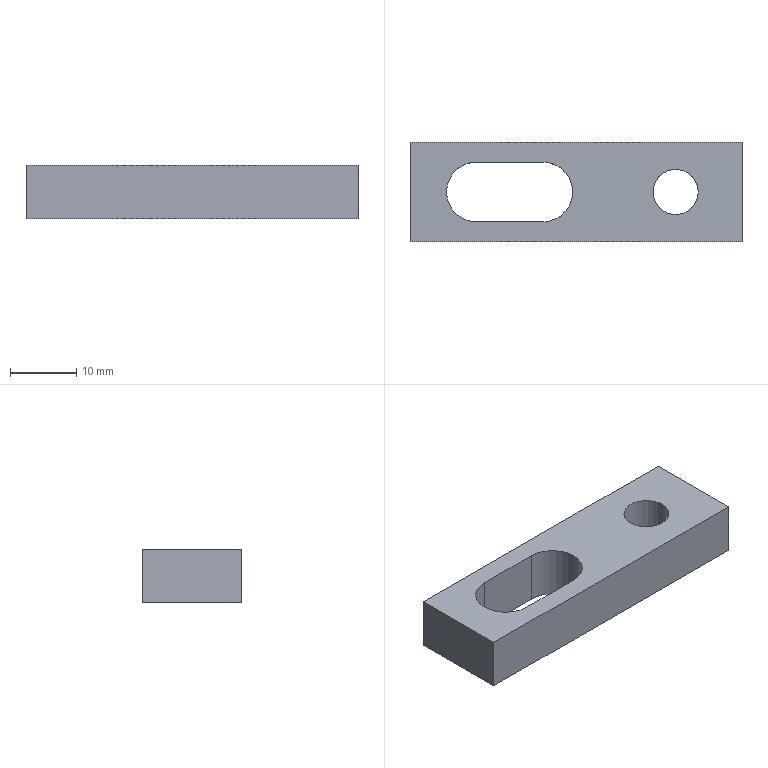Part | STEP file | Tensioning adjustment block QY-1-11 | 1 solid | 13 faces | box 50 x 15 x 8 mm | volume 4481 mm3 | plane 8 | cylinder 5 | commonest cylinder face diameters 9 x3 6.8 x2
STEP:
#1=CARTESIAN_POINT('',(0.,0.,0.));
#2=DIRECTION('',(0.,0.,1.));
#3=DIRECTION('',(1.,0.,0.));
#4=AXIS2_PLACEMENT_3D('',#1,#2,#3);
#5=CARTESIAN_POINT('',(-5.,4.5,0.));
#6=VERTEX_POINT('',#5);
#7=CARTESIAN_POINT('',(-5.,4.5,8.));
#8=VERTEX_POINT('',#7);
#9=CARTESIAN_POINT('',(-5.,4.5,0.));
#10=DIRECTION('',(0.,0.,1.));
#11=VECTOR('',#10,1.);
#12=LINE('',#9,#11);
#13=CARTESIAN_POINT('',(-5.,0.,0.));
#14=DIRECTION('',(0.,0.,1.));
#15=DIRECTION('',(1.,0.,0.));
#16=AXIS2_PLACEMENT_3D('',#13,#14,#15);
#17=CYLINDRICAL_SURFACE('',#16,4.5);
#18=CARTESIAN_POINT('',(1.571,0.));
#19=DIRECTION('',(0.,1.));
#20=VECTOR('',#19,1.);
#21=LINE('',#18,#20);
#22=(GEOMETRIC_REPRESENTATION_CONTEXT(2)PARAMETRIC_REPRESENTATION_CONTEXT()REPRESENTATION_CONTEXT('',''));
#23=DEFINITIONAL_REPRESENTATION('',(#21),#22);
#24=PCURVE('',#17,#23);
#25=CARTESIAN_POINT('',(-15.,4.5,0.));
#26=DIRECTION('',(0.,1.,0.));
#27=DIRECTION('',(-1.,0.,0.));
#28=AXIS2_PLACEMENT_3D('',#25,#26,#27);
#29=PLANE('',#28);
#30=CARTESIAN_POINT('',(-10.,0.));
#31=DIRECTION('',(0.,1.));
#32=VECTOR('',#31,1.);
#33=LINE('',#30,#32);
#34=(GEOMETRIC_REPRESENTATION_CONTEXT(2)PARAMETRIC_REPRESENTATION_CONTEXT()REPRESENTATION_CONTEXT('',''));
#35=DEFINITIONAL_REPRESENTATION('',(#33),#34);
#36=PCURVE('',#29,#35);
#37=SURFACE_CURVE('',#12,(#24,#36),.PCURVE_S1.);
#38=EDGE_CURVE('',#6,#8,#37,.T.);
#39=ORIENTED_EDGE('',*,*,#38,.T.);
#40=CARTESIAN_POINT('',(-0.5,0.,8.));
#41=VERTEX_POINT('',#40);
#42=CARTESIAN_POINT('',(-5.,0.,8.));
#43=DIRECTION('',(0.,0.,1.));
#44=DIRECTION('',(1.,0.,0.));
#45=AXIS2_PLACEMENT_3D('',#42,#43,#44);
#46=CIRCLE('',#45,4.5);
#47=CARTESIAN_POINT('',(0.,8.));
#48=DIRECTION('',(1.,0.));
#49=VECTOR('',#48,1.);
#50=LINE('',#47,#49);
#51=(GEOMETRIC_REPRESENTATION_CONTEXT(2)PARAMETRIC_REPRESENTATION_CONTEXT()REPRESENTATION_CONTEXT('',''));
#52=DEFINITIONAL_REPRESENTATION('',(#50),#51);
#53=PCURVE('',#17,#52);
#54=CARTESIAN_POINT('',(0.,0.,8.));
#55=DIRECTION('',(0.,0.,1.));
#56=DIRECTION('',(1.,0.,0.));
#57=AXIS2_PLACEMENT_3D('',#54,#55,#56);
#58=PLANE('',#57);
#59=CARTESIAN_POINT('',(-5.,0.));
#60=DIRECTION('',(1.,0.));
#61=AXIS2_PLACEMENT_2D('',#59,#60);
#62=CIRCLE('',#61,4.5);
#63=(GEOMETRIC_REPRESENTATION_CONTEXT(2)PARAMETRIC_REPRESENTATION_CONTEXT()REPRESENTATION_CONTEXT('',''));
#64=DEFINITIONAL_REPRESENTATION('',(#62),#63);
#65=PCURVE('',#58,#64);
#66=SURFACE_CURVE('',#46,(#53,#65),.PCURVE_S1.);
#67=EDGE_CURVE('',#41,#8,#66,.T.);
#68=ORIENTED_EDGE('',*,*,#67,.F.);
#69=CARTESIAN_POINT('',(-0.5,0.,0.));
#70=VERTEX_POINT('',#69);
#71=CARTESIAN_POINT('',(-0.5,0.,0.));
#72=DIRECTION('',(0.,0.,1.));
#73=VECTOR('',#72,1.);
#74=LINE('',#71,#73);
#75=CARTESIAN_POINT('',(0.,0.));
#76=DIRECTION('',(0.,1.));
#77=VECTOR('',#76,1.);
#78=LINE('',#75,#77);
#79=(GEOMETRIC_REPRESENTATION_CONTEXT(2)PARAMETRIC_REPRESENTATION_CONTEXT()REPRESENTATION_CONTEXT('',''));
#80=DEFINITIONAL_REPRESENTATION('',(#78),#79);
#81=PCURVE('',#17,#80);
#82=CARTESIAN_POINT('',(-5.,0.,0.));
#83=DIRECTION('',(0.,0.,1.));
#84=DIRECTION('',(1.,0.,0.));
#85=AXIS2_PLACEMENT_3D('',#82,#83,#84);
#86=CYLINDRICAL_SURFACE('',#85,4.5);
#87=CARTESIAN_POINT('',(6.283,0.));
#88=DIRECTION('',(0.,1.));
#89=VECTOR('',#88,1.);
#90=LINE('',#87,#89);
#91=(GEOMETRIC_REPRESENTATION_CONTEXT(2)PARAMETRIC_REPRESENTATION_CONTEXT()REPRESENTATION_CONTEXT('',''));
#92=DEFINITIONAL_REPRESENTATION('',(#90),#91);
#93=PCURVE('',#86,#92);
#94=SURFACE_CURVE('',#74,(#81,#93),.PCURVE_S1.);
#95=EDGE_CURVE('',#70,#41,#94,.T.);
#96=ORIENTED_EDGE('',*,*,#95,.F.);
#97=CARTESIAN_POINT('',(-5.,0.,0.));
#98=DIRECTION('',(0.,0.,1.));
#99=DIRECTION('',(1.,0.,0.));
#100=AXIS2_PLACEMENT_3D('',#97,#98,#99);
#101=CIRCLE('',#100,4.5);
#102=CARTESIAN_POINT('',(0.,0.));
#103=DIRECTION('',(1.,0.));
#104=VECTOR('',#103,1.);
#105=LINE('',#102,#104);
#106=(GEOMETRIC_REPRESENTATION_CONTEXT(2)PARAMETRIC_REPRESENTATION_CONTEXT()REPRESENTATION_CONTEXT('',''));
#107=DEFINITIONAL_REPRESENTATION('',(#105),#106);
#108=PCURVE('',#17,#107);
#109=CARTESIAN_POINT('',(0.,0.,0.));
#110=DIRECTION('',(0.,0.,1.));
#111=DIRECTION('',(1.,0.,0.));
#112=AXIS2_PLACEMENT_3D('',#109,#110,#111);
#113=PLANE('',#112);
#114=CARTESIAN_POINT('',(-5.,0.));
#115=DIRECTION('',(1.,0.));
#116=AXIS2_PLACEMENT_2D('',#114,#115);
#117=CIRCLE('',#116,4.5);
#118=(GEOMETRIC_REPRESENTATION_CONTEXT(2)PARAMETRIC_REPRESENTATION_CONTEXT()REPRESENTATION_CONTEXT('',''));
#119=DEFINITIONAL_REPRESENTATION('',(#117),#118);
#120=PCURVE('',#113,#119);
#121=SURFACE_CURVE('',#101,(#108,#120),.PCURVE_S1.);
#122=EDGE_CURVE('',#70,#6,#121,.T.);
#123=ORIENTED_EDGE('',*,*,#122,.T.);
#124=EDGE_LOOP('',(#39,#68,#96,#123));
#125=FACE_BOUND('',#124,.F.);
#126=ADVANCED_FACE('',(#125),#17,.F.);
#127=CARTESIAN_POINT('',(18.4,0.,0.));
#128=VERTEX_POINT('',#127);
#129=CARTESIAN_POINT('',(18.4,0.,8.));
#130=VERTEX_POINT('',#129);
#131=CARTESIAN_POINT('',(18.4,0.,8.));
#132=DIRECTION('',(0.,0.,1.));
#133=VECTOR('',#132,1.);
#134=LINE('',#131,#133);
#135=CARTESIAN_POINT('',(15.,0.,8.));
#136=DIRECTION('',(0.,0.,1.));
#137=DIRECTION('',(1.,0.,0.));
#138=AXIS2_PLACEMENT_3D('',#135,#136,#137);
#139=CYLINDRICAL_SURFACE('',#138,3.4);
#140=CARTESIAN_POINT('',(6.283,0.));
#141=DIRECTION('',(0.,1.));
#142=VECTOR('',#141,1.);
#143=LINE('',#140,#142);
#144=(GEOMETRIC_REPRESENTATION_CONTEXT(2)PARAMETRIC_REPRESENTATION_CONTEXT()REPRESENTATION_CONTEXT('',''));
#145=DEFINITIONAL_REPRESENTATION('',(#143),#144);
#146=PCURVE('',#139,#145);
#147=CARTESIAN_POINT('',(15.,0.,8.));
#148=DIRECTION('',(0.,0.,1.));
#149=DIRECTION('',(1.,0.,0.));
#150=AXIS2_PLACEMENT_3D('',#147,#148,#149);
#151=CYLINDRICAL_SURFACE('',#150,3.4);
#152=CARTESIAN_POINT('',(0.,0.));
#153=DIRECTION('',(0.,1.));
#154=VECTOR('',#153,1.);
#155=LINE('',#152,#154);
#156=(GEOMETRIC_REPRESENTATION_CONTEXT(2)PARAMETRIC_REPRESENTATION_CONTEXT()REPRESENTATION_CONTEXT('',''));
#157=DEFINITIONAL_REPRESENTATION('',(#155),#156);
#158=PCURVE('',#151,#157);
#159=SURFACE_CURVE('',#134,(#146,#158),.PCURVE_S1.);
#160=EDGE_CURVE('',#128,#130,#159,.T.);
#161=ORIENTED_EDGE('',*,*,#160,.T.);
#162=CARTESIAN_POINT('',(11.6,0.,8.));
#163=VERTEX_POINT('',#162);
#164=CARTESIAN_POINT('',(15.,0.,8.));
#165=DIRECTION('',(0.,0.,1.));
#166=DIRECTION('',(1.,0.,0.));
#167=AXIS2_PLACEMENT_3D('',#164,#165,#166);
#168=CIRCLE('',#167,3.4);
#169=CARTESIAN_POINT('',(0.,0.));
#170=DIRECTION('',(1.,0.));
#171=VECTOR('',#170,1.);
#172=LINE('',#169,#171);
#173=(GEOMETRIC_REPRESENTATION_CONTEXT(2)PARAMETRIC_REPRESENTATION_CONTEXT()REPRESENTATION_CONTEXT('',''));
#174=DEFINITIONAL_REPRESENTATION('',(#172),#173);
#175=PCURVE('',#139,#174);
#176=CARTESIAN_POINT('',(15.,0.));
#177=DIRECTION('',(1.,0.));
#178=AXIS2_PLACEMENT_2D('',#176,#177);
#179=CIRCLE('',#178,3.4);
#180=(GEOMETRIC_REPRESENTATION_CONTEXT(2)PARAMETRIC_REPRESENTATION_CONTEXT()REPRESENTATION_CONTEXT('',''));
#181=DEFINITIONAL_REPRESENTATION('',(#179),#180);
#182=PCURVE('',#58,#181);
#183=SURFACE_CURVE('',#168,(#175,#182),.PCURVE_S1.);
#184=EDGE_CURVE('',#163,#130,#183,.T.);
#185=ORIENTED_EDGE('',*,*,#184,.F.);
#186=CARTESIAN_POINT('',(11.6,0.,0.));
#187=VERTEX_POINT('',#186);
#188=CARTESIAN_POINT('',(11.6,0.,8.));
#189=DIRECTION('',(0.,0.,1.));
#190=VECTOR('',#189,1.);
#191=LINE('',#188,#190);
#192=CARTESIAN_POINT('',(3.142,0.));
#193=DIRECTION('',(0.,1.));
#194=VECTOR('',#193,1.);
#195=LINE('',#192,#194);
#196=(GEOMETRIC_REPRESENTATION_CONTEXT(2)PARAMETRIC_REPRESENTATION_CONTEXT()REPRESENTATION_CONTEXT('',''));
#197=DEFINITIONAL_REPRESENTATION('',(#195),#196);
#198=PCURVE('',#139,#197);
#199=CARTESIAN_POINT('',(3.142,0.));
#200=DIRECTION('',(0.,1.));
#201=VECTOR('',#200,1.);
#202=LINE('',#199,#201);
#203=(GEOMETRIC_REPRESENTATION_CONTEXT(2)PARAMETRIC_REPRESENTATION_CONTEXT()REPRESENTATION_CONTEXT('',''));
#204=DEFINITIONAL_REPRESENTATION('',(#202),#203);
#205=PCURVE('',#151,#204);
#206=SURFACE_CURVE('',#191,(#198,#205),.PCURVE_S1.);
#207=EDGE_CURVE('',#187,#163,#206,.T.);
#208=ORIENTED_EDGE('',*,*,#207,.F.);
#209=CARTESIAN_POINT('',(15.,0.,0.));
#210=DIRECTION('',(0.,0.,1.));
#211=DIRECTION('',(1.,0.,0.));
#212=AXIS2_PLACEMENT_3D('',#209,#210,#211);
#213=CIRCLE('',#212,3.4);
#214=CARTESIAN_POINT('',(0.,-8.));
#215=DIRECTION('',(1.,0.));
#216=VECTOR('',#215,1.);
#217=LINE('',#214,#216);
#218=(GEOMETRIC_REPRESENTATION_CONTEXT(2)PARAMETRIC_REPRESENTATION_CONTEXT()REPRESENTATION_CONTEXT('',''));
#219=DEFINITIONAL_REPRESENTATION('',(#217),#218);
#220=PCURVE('',#139,#219);
#221=CARTESIAN_POINT('',(15.,0.));
#222=DIRECTION('',(1.,0.));
#223=AXIS2_PLACEMENT_2D('',#221,#222);
#224=CIRCLE('',#223,3.4);
#225=(GEOMETRIC_REPRESENTATION_CONTEXT(2)PARAMETRIC_REPRESENTATION_CONTEXT()REPRESENTATION_CONTEXT('',''));
#226=DEFINITIONAL_REPRESENTATION('',(#224),#225);
#227=PCURVE('',#113,#226);
#228=SURFACE_CURVE('',#213,(#220,#227),.PCURVE_S1.);
#229=EDGE_CURVE('',#187,#128,#228,.T.);
#230=ORIENTED_EDGE('',*,*,#229,.T.);
#231=EDGE_LOOP('',(#161,#185,#208,#230));
#232=FACE_BOUND('',#231,.F.);
#233=ADVANCED_FACE('',(#232),#139,.F.);
#234=CARTESIAN_POINT('',(25.,-7.5,0.));
#235=VERTEX_POINT('',#234);
#236=CARTESIAN_POINT('',(25.,7.5,0.));
#237=VERTEX_POINT('',#236);
#238=CARTESIAN_POINT('',(25.,7.5,0.));
#239=DIRECTION('',(0.,1.,0.));
#240=VECTOR('',#239,1.);
#241=LINE('',#238,#240);
#242=CARTESIAN_POINT('',(25.,7.5,8.));
#243=DIRECTION('',(-1.,0.,0.));
#244=DIRECTION('',(0.,0.,1.));
#245=AXIS2_PLACEMENT_3D('',#242,#243,#244);
#246=PLANE('',#245);
#247=CARTESIAN_POINT('',(-8.,0.));
#248=DIRECTION('',(0.,1.));
#249=VECTOR('',#248,1.);
#250=LINE('',#247,#249);
#251=(GEOMETRIC_REPRESENTATION_CONTEXT(2)PARAMETRIC_REPRESENTATION_CONTEXT()REPRESENTATION_CONTEXT('',''));
#252=DEFINITIONAL_REPRESENTATION('',(#250),#251);
#253=PCURVE('',#246,#252);
#254=CARTESIAN_POINT('',(25.,7.5));
#255=DIRECTION('',(0.,1.));
#256=VECTOR('',#255,1.);
#257=LINE('',#254,#256);
#258=(GEOMETRIC_REPRESENTATION_CONTEXT(2)PARAMETRIC_REPRESENTATION_CONTEXT()REPRESENTATION_CONTEXT('',''));
#259=DEFINITIONAL_REPRESENTATION('',(#257),#258);
#260=PCURVE('',#113,#259);
#261=SURFACE_CURVE('',#241,(#253,#260),.PCURVE_S1.);
#262=EDGE_CURVE('',#235,#237,#261,.T.);
#263=ORIENTED_EDGE('',*,*,#262,.T.);
#264=CARTESIAN_POINT('',(25.,7.5,8.));
#265=VERTEX_POINT('',#264);
#266=CARTESIAN_POINT('',(25.,7.5,8.));
#267=DIRECTION('',(0.,0.,-1.));
#268=VECTOR('',#267,1.);
#269=LINE('',#266,#268);
#270=CARTESIAN_POINT('',(0.,0.));
#271=DIRECTION('',(-1.,0.));
#272=VECTOR('',#271,1.);
#273=LINE('',#270,#272);
#274=(GEOMETRIC_REPRESENTATION_CONTEXT(2)PARAMETRIC_REPRESENTATION_CONTEXT()REPRESENTATION_CONTEXT('',''));
#275=DEFINITIONAL_REPRESENTATION('',(#273),#274);
#276=PCURVE('',#246,#275);
#277=CARTESIAN_POINT('',(-25.,7.5,8.));
#278=DIRECTION('',(0.,-1.,0.));
#279=DIRECTION('',(0.,0.,-1.));
#280=AXIS2_PLACEMENT_3D('',#277,#278,#279);
#281=PLANE('',#280);
#282=CARTESIAN_POINT('',(0.,50.));
#283=DIRECTION('',(1.,0.));
#284=VECTOR('',#283,1.);
#285=LINE('',#282,#284);
#286=(GEOMETRIC_REPRESENTATION_CONTEXT(2)PARAMETRIC_REPRESENTATION_CONTEXT()REPRESENTATION_CONTEXT('',''));
#287=DEFINITIONAL_REPRESENTATION('',(#285),#286);
#288=PCURVE('',#281,#287);
#289=SURFACE_CURVE('',#269,(#276,#288),.PCURVE_S1.);
#290=EDGE_CURVE('',#265,#237,#289,.T.);
#291=ORIENTED_EDGE('',*,*,#290,.F.);
#292=CARTESIAN_POINT('',(25.,-7.5,8.));
#293=VERTEX_POINT('',#292);
#294=CARTESIAN_POINT('',(25.,7.5,8.));
#295=DIRECTION('',(0.,1.,0.));
#296=VECTOR('',#295,1.);
#297=LINE('',#294,#296);
#298=CARTESIAN_POINT('',(0.,0.));
#299=DIRECTION('',(0.,1.));
#300=VECTOR('',#299,1.);
#301=LINE('',#298,#300);
#302=(GEOMETRIC_REPRESENTATION_CONTEXT(2)PARAMETRIC_REPRESENTATION_CONTEXT()REPRESENTATION_CONTEXT('',''));
#303=DEFINITIONAL_REPRESENTATION('',(#301),#302);
#304=PCURVE('',#246,#303);
#305=CARTESIAN_POINT('',(25.,7.5));
#306=DIRECTION('',(0.,1.));
#307=VECTOR('',#306,1.);
#308=LINE('',#305,#307);
#309=(GEOMETRIC_REPRESENTATION_CONTEXT(2)PARAMETRIC_REPRESENTATION_CONTEXT()REPRESENTATION_CONTEXT('',''));
#310=DEFINITIONAL_REPRESENTATION('',(#308),#309);
#311=PCURVE('',#58,#310);
#312=SURFACE_CURVE('',#297,(#304,#311),.PCURVE_S1.);
#313=EDGE_CURVE('',#293,#265,#312,.T.);
#314=ORIENTED_EDGE('',*,*,#313,.F.);
#315=CARTESIAN_POINT('',(25.,-7.5,8.));
#316=DIRECTION('',(0.,0.,-1.));
#317=VECTOR('',#316,1.);
#318=LINE('',#315,#317);
#319=CARTESIAN_POINT('',(0.,-15.));
#320=DIRECTION('',(-1.,0.));
#321=VECTOR('',#320,1.);
#322=LINE('',#319,#321);
#323=(GEOMETRIC_REPRESENTATION_CONTEXT(2)PARAMETRIC_REPRESENTATION_CONTEXT()REPRESENTATION_CONTEXT('',''));
#324=DEFINITIONAL_REPRESENTATION('',(#322),#323);
#325=PCURVE('',#246,#324);
#326=CARTESIAN_POINT('',(-25.,-7.5,8.));
#327=DIRECTION('',(0.,1.,0.));
#328=DIRECTION('',(0.,0.,1.));
#329=AXIS2_PLACEMENT_3D('',#326,#327,#328);
#330=PLANE('',#329);
#331=CARTESIAN_POINT('',(0.,50.));
#332=DIRECTION('',(-1.,0.));
#333=VECTOR('',#332,1.);
#334=LINE('',#331,#333);
#335=(GEOMETRIC_REPRESENTATION_CONTEXT(2)PARAMETRIC_REPRESENTATION_CONTEXT()REPRESENTATION_CONTEXT('',''));
#336=DEFINITIONAL_REPRESENTATION('',(#334),#335);
#337=PCURVE('',#330,#336);
#338=SURFACE_CURVE('',#318,(#325,#337),.PCURVE_S1.);
#339=EDGE_CURVE('',#293,#235,#338,.T.);
#340=ORIENTED_EDGE('',*,*,#339,.T.);
#341=EDGE_LOOP('',(#263,#291,#314,#340));
#342=FACE_BOUND('',#341,.T.);
#343=ADVANCED_FACE('',(#342),#246,.F.);
#344=CARTESIAN_POINT('',(-25.,7.5,0.));
#345=VERTEX_POINT('',#344);
#346=CARTESIAN_POINT('',(-25.,7.5,0.));
#347=DIRECTION('',(-1.,0.,0.));
#348=VECTOR('',#347,1.);
#349=LINE('',#346,#348);
#350=CARTESIAN_POINT('',(8.,0.));
#351=DIRECTION('',(0.,-1.));
#352=VECTOR('',#351,1.);
#353=LINE('',#350,#352);
#354=(GEOMETRIC_REPRESENTATION_CONTEXT(2)PARAMETRIC_REPRESENTATION_CONTEXT()REPRESENTATION_CONTEXT('',''));
#355=DEFINITIONAL_REPRESENTATION('',(#353),#354);
#356=PCURVE('',#281,#355);
#357=CARTESIAN_POINT('',(-25.,7.5));
#358=DIRECTION('',(-1.,0.));
#359=VECTOR('',#358,1.);
#360=LINE('',#357,#359);
#361=(GEOMETRIC_REPRESENTATION_CONTEXT(2)PARAMETRIC_REPRESENTATION_CONTEXT()REPRESENTATION_CONTEXT('',''));
#362=DEFINITIONAL_REPRESENTATION('',(#360),#361);
#363=PCURVE('',#113,#362);
#364=SURFACE_CURVE('',#349,(#356,#363),.PCURVE_S1.);
#365=EDGE_CURVE('',#237,#345,#364,.T.);
#366=ORIENTED_EDGE('',*,*,#365,.T.);
#367=CARTESIAN_POINT('',(-25.,7.5,8.));
#368=VERTEX_POINT('',#367);
#369=CARTESIAN_POINT('',(-25.,7.5,8.));
#370=DIRECTION('',(0.,0.,-1.));
#371=VECTOR('',#370,1.);
#372=LINE('',#369,#371);
#373=CARTESIAN_POINT('',(0.,0.));
#374=DIRECTION('',(1.,0.));
#375=VECTOR('',#374,1.);
#376=LINE('',#373,#375);
#377=(GEOMETRIC_REPRESENTATION_CONTEXT(2)PARAMETRIC_REPRESENTATION_CONTEXT()REPRESENTATION_CONTEXT('',''));
#378=DEFINITIONAL_REPRESENTATION('',(#376),#377);
#379=PCURVE('',#281,#378);
#380=CARTESIAN_POINT('',(-25.,7.5,8.));
#381=DIRECTION('',(1.,0.,0.));
#382=DIRECTION('',(0.,0.,-1.));
#383=AXIS2_PLACEMENT_3D('',#380,#381,#382);
#384=PLANE('',#383);
#385=CARTESIAN_POINT('',(0.,0.));
#386=DIRECTION('',(1.,0.));
#387=VECTOR('',#386,1.);
#388=LINE('',#385,#387);
#389=(GEOMETRIC_REPRESENTATION_CONTEXT(2)PARAMETRIC_REPRESENTATION_CONTEXT()REPRESENTATION_CONTEXT('',''));
#390=DEFINITIONAL_REPRESENTATION('',(#388),#389);
#391=PCURVE('',#384,#390);
#392=SURFACE_CURVE('',#372,(#379,#391),.PCURVE_S1.);
#393=EDGE_CURVE('',#368,#345,#392,.T.);
#394=ORIENTED_EDGE('',*,*,#393,.F.);
#395=CARTESIAN_POINT('',(-25.,7.5,8.));
#396=DIRECTION('',(-1.,0.,0.));
#397=VECTOR('',#396,1.);
#398=LINE('',#395,#397);
#399=CARTESIAN_POINT('',(0.,0.));
#400=DIRECTION('',(0.,-1.));
#401=VECTOR('',#400,1.);
#402=LINE('',#399,#401);
#403=(GEOMETRIC_REPRESENTATION_CONTEXT(2)PARAMETRIC_REPRESENTATION_CONTEXT()REPRESENTATION_CONTEXT('',''));
#404=DEFINITIONAL_REPRESENTATION('',(#402),#403);
#405=PCURVE('',#281,#404);
#406=CARTESIAN_POINT('',(-25.,7.5));
#407=DIRECTION('',(-1.,0.));
#408=VECTOR('',#407,1.);
#409=LINE('',#406,#408);
#410=(GEOMETRIC_REPRESENTATION_CONTEXT(2)PARAMETRIC_REPRESENTATION_CONTEXT()REPRESENTATION_CONTEXT('',''));
#411=DEFINITIONAL_REPRESENTATION('',(#409),#410);
#412=PCURVE('',#58,#411);
#413=SURFACE_CURVE('',#398,(#405,#412),.PCURVE_S1.);
#414=EDGE_CURVE('',#265,#368,#413,.T.);
#415=ORIENTED_EDGE('',*,*,#414,.F.);
#416=ORIENTED_EDGE('',*,*,#290,.T.);
#417=EDGE_LOOP('',(#366,#394,#415,#416));
#418=FACE_BOUND('',#417,.T.);
#419=ADVANCED_FACE('',(#418),#281,.F.);
#420=CARTESIAN_POINT('',(-25.,-7.5,0.));
#421=VERTEX_POINT('',#420);
#422=CARTESIAN_POINT('',(-25.,7.5,0.));
#423=DIRECTION('',(0.,-1.,0.));
#424=VECTOR('',#423,1.);
#425=LINE('',#422,#424);
#426=CARTESIAN_POINT('',(8.,0.));
#427=DIRECTION('',(0.,-1.));
#428=VECTOR('',#427,1.);
#429=LINE('',#426,#428);
#430=(GEOMETRIC_REPRESENTATION_CONTEXT(2)PARAMETRIC_REPRESENTATION_CONTEXT()REPRESENTATION_CONTEXT('',''));
#431=DEFINITIONAL_REPRESENTATION('',(#429),#430);
#432=PCURVE('',#384,#431);
#433=CARTESIAN_POINT('',(-25.,7.5));
#434=DIRECTION('',(0.,-1.));
#435=VECTOR('',#434,1.);
#436=LINE('',#433,#435);
#437=(GEOMETRIC_REPRESENTATION_CONTEXT(2)PARAMETRIC_REPRESENTATION_CONTEXT()REPRESENTATION_CONTEXT('',''));
#438=DEFINITIONAL_REPRESENTATION('',(#436),#437);
#439=PCURVE('',#113,#438);
#440=SURFACE_CURVE('',#425,(#432,#439),.PCURVE_S1.);
#441=EDGE_CURVE('',#345,#421,#440,.T.);
#442=ORIENTED_EDGE('',*,*,#441,.T.);
#443=CARTESIAN_POINT('',(-25.,-7.5,8.));
#444=VERTEX_POINT('',#443);
#445=CARTESIAN_POINT('',(-25.,-7.5,8.));
#446=DIRECTION('',(0.,0.,-1.));
#447=VECTOR('',#446,1.);
#448=LINE('',#445,#447);
#449=CARTESIAN_POINT('',(0.,-15.));
#450=DIRECTION('',(1.,0.));
#451=VECTOR('',#450,1.);
#452=LINE('',#449,#451);
#453=(GEOMETRIC_REPRESENTATION_CONTEXT(2)PARAMETRIC_REPRESENTATION_CONTEXT()REPRESENTATION_CONTEXT('',''));
#454=DEFINITIONAL_REPRESENTATION('',(#452),#453);
#455=PCURVE('',#384,#454);
#456=CARTESIAN_POINT('',(0.,0.));
#457=DIRECTION('',(-1.,0.));
#458=VECTOR('',#457,1.);
#459=LINE('',#456,#458);
#460=(GEOMETRIC_REPRESENTATION_CONTEXT(2)PARAMETRIC_REPRESENTATION_CONTEXT()REPRESENTATION_CONTEXT('',''));
#461=DEFINITIONAL_REPRESENTATION('',(#459),#460);
#462=PCURVE('',#330,#461);
#463=SURFACE_CURVE('',#448,(#455,#462),.PCURVE_S1.);
#464=EDGE_CURVE('',#444,#421,#463,.T.);
#465=ORIENTED_EDGE('',*,*,#464,.F.);
#466=CARTESIAN_POINT('',(-25.,7.5,8.));
#467=DIRECTION('',(0.,-1.,0.));
#468=VECTOR('',#467,1.);
#469=LINE('',#466,#468);
#470=CARTESIAN_POINT('',(0.,0.));
#471=DIRECTION('',(0.,-1.));
#472=VECTOR('',#471,1.);
#473=LINE('',#470,#472);
#474=(GEOMETRIC_REPRESENTATION_CONTEXT(2)PARAMETRIC_REPRESENTATION_CONTEXT()REPRESENTATION_CONTEXT('',''));
#475=DEFINITIONAL_REPRESENTATION('',(#473),#474);
#476=PCURVE('',#384,#475);
#477=CARTESIAN_POINT('',(-25.,7.5));
#478=DIRECTION('',(0.,-1.));
#479=VECTOR('',#478,1.);
#480=LINE('',#477,#479);
#481=(GEOMETRIC_REPRESENTATION_CONTEXT(2)PARAMETRIC_REPRESENTATION_CONTEXT()REPRESENTATION_CONTEXT('',''));
#482=DEFINITIONAL_REPRESENTATION('',(#480),#481);
#483=PCURVE('',#58,#482);
#484=SURFACE_CURVE('',#469,(#476,#483),.PCURVE_S1.);
#485=EDGE_CURVE('',#368,#444,#484,.T.);
#486=ORIENTED_EDGE('',*,*,#485,.F.);
#487=ORIENTED_EDGE('',*,*,#393,.T.);
#488=EDGE_LOOP('',(#442,#465,#486,#487));
#489=FACE_BOUND('',#488,.T.);
#490=ADVANCED_FACE('',(#489),#384,.F.);
#491=CARTESIAN_POINT('',(-25.,-7.5,0.));
#492=DIRECTION('',(1.,0.,0.));
#493=VECTOR('',#492,1.);
#494=LINE('',#491,#493);
#495=CARTESIAN_POINT('',(-8.,0.));
#496=DIRECTION('',(0.,1.));
#497=VECTOR('',#496,1.);
#498=LINE('',#495,#497);
#499=(GEOMETRIC_REPRESENTATION_CONTEXT(2)PARAMETRIC_REPRESENTATION_CONTEXT()REPRESENTATION_CONTEXT('',''));
#500=DEFINITIONAL_REPRESENTATION('',(#498),#499);
#501=PCURVE('',#330,#500);
#502=CARTESIAN_POINT('',(-25.,-7.5));
#503=DIRECTION('',(1.,0.));
#504=VECTOR('',#503,1.);
#505=LINE('',#502,#504);
#506=(GEOMETRIC_REPRESENTATION_CONTEXT(2)PARAMETRIC_REPRESENTATION_CONTEXT()REPRESENTATION_CONTEXT('',''));
#507=DEFINITIONAL_REPRESENTATION('',(#505),#506);
#508=PCURVE('',#113,#507);
#509=SURFACE_CURVE('',#494,(#501,#508),.PCURVE_S1.);
#510=EDGE_CURVE('',#421,#235,#509,.T.);
#511=ORIENTED_EDGE('',*,*,#510,.T.);
#512=ORIENTED_EDGE('',*,*,#339,.F.);
#513=CARTESIAN_POINT('',(-25.,-7.5,8.));
#514=DIRECTION('',(1.,0.,0.));
#515=VECTOR('',#514,1.);
#516=LINE('',#513,#515);
#517=CARTESIAN_POINT('',(0.,0.));
#518=DIRECTION('',(0.,1.));
#519=VECTOR('',#518,1.);
#520=LINE('',#517,#519);
#521=(GEOMETRIC_REPRESENTATION_CONTEXT(2)PARAMETRIC_REPRESENTATION_CONTEXT()REPRESENTATION_CONTEXT('',''));
#522=DEFINITIONAL_REPRESENTATION('',(#520),#521);
#523=PCURVE('',#330,#522);
#524=CARTESIAN_POINT('',(-25.,-7.5));
#525=DIRECTION('',(1.,0.));
#526=VECTOR('',#525,1.);
#527=LINE('',#524,#526);
#528=(GEOMETRIC_REPRESENTATION_CONTEXT(2)PARAMETRIC_REPRESENTATION_CONTEXT()REPRESENTATION_CONTEXT('',''));
#529=DEFINITIONAL_REPRESENTATION('',(#527),#528);
#530=PCURVE('',#58,#529);
#531=SURFACE_CURVE('',#516,(#523,#530),.PCURVE_S1.);
#532=EDGE_CURVE('',#444,#293,#531,.T.);
#533=ORIENTED_EDGE('',*,*,#532,.F.);
#534=ORIENTED_EDGE('',*,*,#464,.T.);
#535=EDGE_LOOP('',(#511,#512,#533,#534));
#536=FACE_BOUND('',#535,.T.);
#537=ADVANCED_FACE('',(#536),#330,.F.);
#538=CARTESIAN_POINT('',(-15.,4.5,8.));
#539=VERTEX_POINT('',#538);
#540=CARTESIAN_POINT('',(-15.,-4.5,8.));
#541=VERTEX_POINT('',#540);
#542=CARTESIAN_POINT('',(-15.,0.,8.));
#543=DIRECTION('',(0.,0.,1.));
#544=DIRECTION('',(1.,0.,0.));
#545=AXIS2_PLACEMENT_3D('',#542,#543,#544);
#546=CIRCLE('',#545,4.5);
#547=CARTESIAN_POINT('',(-15.,0.));
#548=DIRECTION('',(1.,0.));
#549=AXIS2_PLACEMENT_2D('',#547,#548);
#550=CIRCLE('',#549,4.5);
#551=(GEOMETRIC_REPRESENTATION_CONTEXT(2)PARAMETRIC_REPRESENTATION_CONTEXT()REPRESENTATION_CONTEXT('',''));
#552=DEFINITIONAL_REPRESENTATION('',(#550),#551);
#553=PCURVE('',#58,#552);
#554=CARTESIAN_POINT('',(-15.,0.,0.));
#555=DIRECTION('',(0.,0.,1.));
#556=DIRECTION('',(1.,0.,0.));
#557=AXIS2_PLACEMENT_3D('',#554,#555,#556);
#558=CYLINDRICAL_SURFACE('',#557,4.5);
#559=CARTESIAN_POINT('',(0.,8.));
#560=DIRECTION('',(1.,0.));
#561=VECTOR('',#560,1.);
#562=LINE('',#559,#561);
#563=(GEOMETRIC_REPRESENTATION_CONTEXT(2)PARAMETRIC_REPRESENTATION_CONTEXT()REPRESENTATION_CONTEXT('',''));
#564=DEFINITIONAL_REPRESENTATION('',(#562),#563);
#565=PCURVE('',#558,#564);
#566=SURFACE_CURVE('',#546,(#553,#565),.PCURVE_S1.);
#567=EDGE_CURVE('',#539,#541,#566,.T.);
#568=ORIENTED_EDGE('',*,*,#567,.F.);
#569=CARTESIAN_POINT('',(-15.,4.5,8.));
#570=DIRECTION('',(-1.,0.,0.));
#571=VECTOR('',#570,1.);
#572=LINE('',#569,#571);
#573=CARTESIAN_POINT('',(-15.,4.5));
#574=DIRECTION('',(-1.,0.));
#575=VECTOR('',#574,1.);
#576=LINE('',#573,#575);
#577=(GEOMETRIC_REPRESENTATION_CONTEXT(2)PARAMETRIC_REPRESENTATION_CONTEXT()REPRESENTATION_CONTEXT('',''));
#578=DEFINITIONAL_REPRESENTATION('',(#576),#577);
#579=PCURVE('',#58,#578);
#580=CARTESIAN_POINT('',(0.,8.));
#581=DIRECTION('',(1.,0.));
#582=VECTOR('',#581,1.);
#583=LINE('',#580,#582);
#584=(GEOMETRIC_REPRESENTATION_CONTEXT(2)PARAMETRIC_REPRESENTATION_CONTEXT()REPRESENTATION_CONTEXT('',''));
#585=DEFINITIONAL_REPRESENTATION('',(#583),#584);
#586=PCURVE('',#29,#585);
#587=SURFACE_CURVE('',#572,(#579,#586),.PCURVE_S1.);
#588=EDGE_CURVE('',#8,#539,#587,.T.);
#589=ORIENTED_EDGE('',*,*,#588,.F.);
#590=ORIENTED_EDGE('',*,*,#67,.F.);
#591=CARTESIAN_POINT('',(-5.,-4.5,8.));
#592=VERTEX_POINT('',#591);
#593=CARTESIAN_POINT('',(-5.,0.,8.));
#594=DIRECTION('',(0.,0.,1.));
#595=DIRECTION('',(1.,0.,0.));
#596=AXIS2_PLACEMENT_3D('',#593,#594,#595);
#597=CIRCLE('',#596,4.5);
#598=CARTESIAN_POINT('',(-5.,0.));
#599=DIRECTION('',(1.,0.));
#600=AXIS2_PLACEMENT_2D('',#598,#599);
#601=CIRCLE('',#600,4.5);
#602=(GEOMETRIC_REPRESENTATION_CONTEXT(2)PARAMETRIC_REPRESENTATION_CONTEXT()REPRESENTATION_CONTEXT('',''));
#603=DEFINITIONAL_REPRESENTATION('',(#601),#602);
#604=PCURVE('',#58,#603);
#605=CARTESIAN_POINT('',(0.,8.));
#606=DIRECTION('',(1.,0.));
#607=VECTOR('',#606,1.);
#608=LINE('',#605,#607);
#609=(GEOMETRIC_REPRESENTATION_CONTEXT(2)PARAMETRIC_REPRESENTATION_CONTEXT()REPRESENTATION_CONTEXT('',''));
#610=DEFINITIONAL_REPRESENTATION('',(#608),#609);
#611=PCURVE('',#86,#610);
#612=SURFACE_CURVE('',#597,(#604,#611),.PCURVE_S1.);
#613=EDGE_CURVE('',#592,#41,#612,.T.);
#614=ORIENTED_EDGE('',*,*,#613,.F.);
#615=CARTESIAN_POINT('',(-15.,-4.5,8.));
#616=DIRECTION('',(1.,0.,0.));
#617=VECTOR('',#616,1.);
#618=LINE('',#615,#617);
#619=CARTESIAN_POINT('',(-15.,-4.5));
#620=DIRECTION('',(1.,0.));
#621=VECTOR('',#620,1.);
#622=LINE('',#619,#621);
#623=(GEOMETRIC_REPRESENTATION_CONTEXT(2)PARAMETRIC_REPRESENTATION_CONTEXT()REPRESENTATION_CONTEXT('',''));
#624=DEFINITIONAL_REPRESENTATION('',(#622),#623);
#625=PCURVE('',#58,#624);
#626=CARTESIAN_POINT('',(-15.,-4.5,0.));
#627=DIRECTION('',(0.,-1.,0.));
#628=DIRECTION('',(1.,0.,0.));
#629=AXIS2_PLACEMENT_3D('',#626,#627,#628);
#630=PLANE('',#629);
#631=CARTESIAN_POINT('',(0.,8.));
#632=DIRECTION('',(1.,0.));
#633=VECTOR('',#632,1.);
#634=LINE('',#631,#633);
#635=(GEOMETRIC_REPRESENTATION_CONTEXT(2)PARAMETRIC_REPRESENTATION_CONTEXT()REPRESENTATION_CONTEXT('',''));
#636=DEFINITIONAL_REPRESENTATION('',(#634),#635);
#637=PCURVE('',#630,#636);
#638=SURFACE_CURVE('',#618,(#625,#637),.PCURVE_S1.);
#639=EDGE_CURVE('',#541,#592,#638,.T.);
#640=ORIENTED_EDGE('',*,*,#639,.F.);
#641=EDGE_LOOP('',(#568,#589,#590,#614,#640));
#642=FACE_BOUND('',#641,.T.);
#643=CARTESIAN_POINT('',(15.,0.,8.));
#644=DIRECTION('',(0.,0.,1.));
#645=DIRECTION('',(1.,0.,0.));
#646=AXIS2_PLACEMENT_3D('',#643,#644,#645);
#647=CIRCLE('',#646,3.4);
#648=CARTESIAN_POINT('',(15.,0.));
#649=DIRECTION('',(1.,0.));
#650=AXIS2_PLACEMENT_2D('',#648,#649);
#651=CIRCLE('',#650,3.4);
#652=(GEOMETRIC_REPRESENTATION_CONTEXT(2)PARAMETRIC_REPRESENTATION_CONTEXT()REPRESENTATION_CONTEXT('',''));
#653=DEFINITIONAL_REPRESENTATION('',(#651),#652);
#654=PCURVE('',#58,#653);
#655=CARTESIAN_POINT('',(0.,0.));
#656=DIRECTION('',(1.,0.));
#657=VECTOR('',#656,1.);
#658=LINE('',#655,#657);
#659=(GEOMETRIC_REPRESENTATION_CONTEXT(2)PARAMETRIC_REPRESENTATION_CONTEXT()REPRESENTATION_CONTEXT('',''));
#660=DEFINITIONAL_REPRESENTATION('',(#658),#659);
#661=PCURVE('',#151,#660);
#662=SURFACE_CURVE('',#647,(#654,#661),.PCURVE_S1.);
#663=EDGE_CURVE('',#130,#163,#662,.T.);
#664=ORIENTED_EDGE('',*,*,#663,.F.);
#665=ORIENTED_EDGE('',*,*,#184,.F.);
#666=EDGE_LOOP('',(#664,#665));
#667=FACE_BOUND('',#666,.T.);
#668=ORIENTED_EDGE('',*,*,#313,.T.);
#669=ORIENTED_EDGE('',*,*,#414,.T.);
#670=ORIENTED_EDGE('',*,*,#485,.T.);
#671=ORIENTED_EDGE('',*,*,#532,.T.);
#672=EDGE_LOOP('',(#668,#669,#670,#671));
#673=FACE_BOUND('',#672,.T.);
#674=ADVANCED_FACE('',(#642,#667,#673),#58,.T.);
#675=CARTESIAN_POINT('',(-15.,4.5,0.));
#676=VERTEX_POINT('',#675);
#677=CARTESIAN_POINT('',(-15.,4.5,0.));
#678=DIRECTION('',(-1.,0.,0.));
#679=VECTOR('',#678,1.);
#680=LINE('',#677,#679);
#681=CARTESIAN_POINT('',(-15.,4.5));
#682=DIRECTION('',(-1.,0.));
#683=VECTOR('',#682,1.);
#684=LINE('',#681,#683);
#685=(GEOMETRIC_REPRESENTATION_CONTEXT(2)PARAMETRIC_REPRESENTATION_CONTEXT()REPRESENTATION_CONTEXT('',''));
#686=DEFINITIONAL_REPRESENTATION('',(#684),#685);
#687=PCURVE('',#113,#686);
#688=CARTESIAN_POINT('',(0.,0.));
#689=DIRECTION('',(1.,0.));
#690=VECTOR('',#689,1.);
#691=LINE('',#688,#690);
#692=(GEOMETRIC_REPRESENTATION_CONTEXT(2)PARAMETRIC_REPRESENTATION_CONTEXT()REPRESENTATION_CONTEXT('',''));
#693=DEFINITIONAL_REPRESENTATION('',(#691),#692);
#694=PCURVE('',#29,#693);
#695=SURFACE_CURVE('',#680,(#687,#694),.PCURVE_S1.);
#696=EDGE_CURVE('',#6,#676,#695,.T.);
#697=ORIENTED_EDGE('',*,*,#696,.T.);
#698=CARTESIAN_POINT('',(-15.,-4.5,0.));
#699=VERTEX_POINT('',#698);
#700=CARTESIAN_POINT('',(-15.,0.,0.));
#701=DIRECTION('',(0.,0.,1.));
#702=DIRECTION('',(1.,0.,0.));
#703=AXIS2_PLACEMENT_3D('',#700,#701,#702);
#704=CIRCLE('',#703,4.5);
#705=CARTESIAN_POINT('',(-15.,0.));
#706=DIRECTION('',(1.,0.));
#707=AXIS2_PLACEMENT_2D('',#705,#706);
#708=CIRCLE('',#707,4.5);
#709=(GEOMETRIC_REPRESENTATION_CONTEXT(2)PARAMETRIC_REPRESENTATION_CONTEXT()REPRESENTATION_CONTEXT('',''));
#710=DEFINITIONAL_REPRESENTATION('',(#708),#709);
#711=PCURVE('',#113,#710);
#712=CARTESIAN_POINT('',(0.,0.));
#713=DIRECTION('',(1.,0.));
#714=VECTOR('',#713,1.);
#715=LINE('',#712,#714);
#716=(GEOMETRIC_REPRESENTATION_CONTEXT(2)PARAMETRIC_REPRESENTATION_CONTEXT()REPRESENTATION_CONTEXT('',''));
#717=DEFINITIONAL_REPRESENTATION('',(#715),#716);
#718=PCURVE('',#558,#717);
#719=SURFACE_CURVE('',#704,(#711,#718),.PCURVE_S1.);
#720=EDGE_CURVE('',#676,#699,#719,.T.);
#721=ORIENTED_EDGE('',*,*,#720,.T.);
#722=CARTESIAN_POINT('',(-5.,-4.5,0.));
#723=VERTEX_POINT('',#722);
#724=CARTESIAN_POINT('',(-15.,-4.5,0.));
#725=DIRECTION('',(1.,0.,0.));
#726=VECTOR('',#725,1.);
#727=LINE('',#724,#726);
#728=CARTESIAN_POINT('',(-15.,-4.5));
#729=DIRECTION('',(1.,0.));
#730=VECTOR('',#729,1.);
#731=LINE('',#728,#730);
#732=(GEOMETRIC_REPRESENTATION_CONTEXT(2)PARAMETRIC_REPRESENTATION_CONTEXT()REPRESENTATION_CONTEXT('',''));
#733=DEFINITIONAL_REPRESENTATION('',(#731),#732);
#734=PCURVE('',#113,#733);
#735=CARTESIAN_POINT('',(0.,0.));
#736=DIRECTION('',(1.,0.));
#737=VECTOR('',#736,1.);
#738=LINE('',#735,#737);
#739=(GEOMETRIC_REPRESENTATION_CONTEXT(2)PARAMETRIC_REPRESENTATION_CONTEXT()REPRESENTATION_CONTEXT('',''));
#740=DEFINITIONAL_REPRESENTATION('',(#738),#739);
#741=PCURVE('',#630,#740);
#742=SURFACE_CURVE('',#727,(#734,#741),.PCURVE_S1.);
#743=EDGE_CURVE('',#699,#723,#742,.T.);
#744=ORIENTED_EDGE('',*,*,#743,.T.);
#745=CARTESIAN_POINT('',(-5.,0.,0.));
#746=DIRECTION('',(0.,0.,1.));
#747=DIRECTION('',(1.,0.,0.));
#748=AXIS2_PLACEMENT_3D('',#745,#746,#747);
#749=CIRCLE('',#748,4.5);
#750=CARTESIAN_POINT('',(-5.,0.));
#751=DIRECTION('',(1.,0.));
#752=AXIS2_PLACEMENT_2D('',#750,#751);
#753=CIRCLE('',#752,4.5);
#754=(GEOMETRIC_REPRESENTATION_CONTEXT(2)PARAMETRIC_REPRESENTATION_CONTEXT()REPRESENTATION_CONTEXT('',''));
#755=DEFINITIONAL_REPRESENTATION('',(#753),#754);
#756=PCURVE('',#113,#755);
#757=CARTESIAN_POINT('',(0.,0.));
#758=DIRECTION('',(1.,0.));
#759=VECTOR('',#758,1.);
#760=LINE('',#757,#759);
#761=(GEOMETRIC_REPRESENTATION_CONTEXT(2)PARAMETRIC_REPRESENTATION_CONTEXT()REPRESENTATION_CONTEXT('',''));
#762=DEFINITIONAL_REPRESENTATION('',(#760),#761);
#763=PCURVE('',#86,#762);
#764=SURFACE_CURVE('',#749,(#756,#763),.PCURVE_S1.);
#765=EDGE_CURVE('',#723,#70,#764,.T.);
#766=ORIENTED_EDGE('',*,*,#765,.T.);
#767=ORIENTED_EDGE('',*,*,#122,.T.);
#768=EDGE_LOOP('',(#697,#721,#744,#766,#767));
#769=FACE_BOUND('',#768,.T.);
#770=CARTESIAN_POINT('',(15.,0.,0.));
#771=DIRECTION('',(0.,0.,1.));
#772=DIRECTION('',(1.,0.,0.));
#773=AXIS2_PLACEMENT_3D('',#770,#771,#772);
#774=CIRCLE('',#773,3.4);
#775=CARTESIAN_POINT('',(15.,0.));
#776=DIRECTION('',(1.,0.));
#777=AXIS2_PLACEMENT_2D('',#775,#776);
#778=CIRCLE('',#777,3.4);
#779=(GEOMETRIC_REPRESENTATION_CONTEXT(2)PARAMETRIC_REPRESENTATION_CONTEXT()REPRESENTATION_CONTEXT('',''));
#780=DEFINITIONAL_REPRESENTATION('',(#778),#779);
#781=PCURVE('',#113,#780);
#782=CARTESIAN_POINT('',(0.,-8.));
#783=DIRECTION('',(1.,0.));
#784=VECTOR('',#783,1.);
#785=LINE('',#782,#784);
#786=(GEOMETRIC_REPRESENTATION_CONTEXT(2)PARAMETRIC_REPRESENTATION_CONTEXT()REPRESENTATION_CONTEXT('',''));
#787=DEFINITIONAL_REPRESENTATION('',(#785),#786);
#788=PCURVE('',#151,#787);
#789=SURFACE_CURVE('',#774,(#781,#788),.PCURVE_S1.);
#790=EDGE_CURVE('',#128,#187,#789,.T.);
#791=ORIENTED_EDGE('',*,*,#790,.T.);
#792=ORIENTED_EDGE('',*,*,#229,.T.);
#793=EDGE_LOOP('',(#791,#792));
#794=FACE_BOUND('',#793,.T.);
#795=ORIENTED_EDGE('',*,*,#262,.F.);
#796=ORIENTED_EDGE('',*,*,#510,.F.);
#797=ORIENTED_EDGE('',*,*,#441,.F.);
#798=ORIENTED_EDGE('',*,*,#365,.F.);
#799=EDGE_LOOP('',(#795,#796,#797,#798));
#800=FACE_BOUND('',#799,.T.);
#801=ADVANCED_FACE('',(#769,#794,#800),#113,.F.);
#802=ORIENTED_EDGE('',*,*,#663,.F.);
#803=ORIENTED_EDGE('',*,*,#160,.F.);
#804=ORIENTED_EDGE('',*,*,#790,.T.);
#805=ORIENTED_EDGE('',*,*,#207,.T.);
#806=EDGE_LOOP('',(#802,#803,#804,#805));
#807=FACE_BOUND('',#806,.F.);
#808=ADVANCED_FACE('',(#807),#151,.F.);
#809=CARTESIAN_POINT('',(-15.,4.5,0.));
#810=DIRECTION('',(0.,0.,1.));
#811=VECTOR('',#810,1.);
#812=LINE('',#809,#811);
#813=CARTESIAN_POINT('',(1.571,0.));
#814=DIRECTION('',(0.,1.));
#815=VECTOR('',#814,1.);
#816=LINE('',#813,#815);
#817=(GEOMETRIC_REPRESENTATION_CONTEXT(2)PARAMETRIC_REPRESENTATION_CONTEXT()REPRESENTATION_CONTEXT('',''));
#818=DEFINITIONAL_REPRESENTATION('',(#816),#817);
#819=PCURVE('',#558,#818);
#820=CARTESIAN_POINT('',(0.,0.));
#821=DIRECTION('',(0.,1.));
#822=VECTOR('',#821,1.);
#823=LINE('',#820,#822);
#824=(GEOMETRIC_REPRESENTATION_CONTEXT(2)PARAMETRIC_REPRESENTATION_CONTEXT()REPRESENTATION_CONTEXT('',''));
#825=DEFINITIONAL_REPRESENTATION('',(#823),#824);
#826=PCURVE('',#29,#825);
#827=SURFACE_CURVE('',#812,(#819,#826),.PCURVE_S1.);
#828=EDGE_CURVE('',#676,#539,#827,.T.);
#829=ORIENTED_EDGE('',*,*,#828,.F.);
#830=ORIENTED_EDGE('',*,*,#720,.T.);
#831=CARTESIAN_POINT('',(-15.,-4.5,0.));
#832=DIRECTION('',(0.,0.,1.));
#833=VECTOR('',#832,1.);
#834=LINE('',#831,#833);
#835=CARTESIAN_POINT('',(4.712,0.));
#836=DIRECTION('',(0.,1.));
#837=VECTOR('',#836,1.);
#838=LINE('',#835,#837);
#839=(GEOMETRIC_REPRESENTATION_CONTEXT(2)PARAMETRIC_REPRESENTATION_CONTEXT()REPRESENTATION_CONTEXT('',''));
#840=DEFINITIONAL_REPRESENTATION('',(#838),#839);
#841=PCURVE('',#558,#840);
#842=CARTESIAN_POINT('',(0.,0.));
#843=DIRECTION('',(0.,1.));
#844=VECTOR('',#843,1.);
#845=LINE('',#842,#844);
#846=(GEOMETRIC_REPRESENTATION_CONTEXT(2)PARAMETRIC_REPRESENTATION_CONTEXT()REPRESENTATION_CONTEXT('',''));
#847=DEFINITIONAL_REPRESENTATION('',(#845),#846);
#848=PCURVE('',#630,#847);
#849=SURFACE_CURVE('',#834,(#841,#848),.PCURVE_S1.);
#850=EDGE_CURVE('',#699,#541,#849,.T.);
#851=ORIENTED_EDGE('',*,*,#850,.T.);
#852=ORIENTED_EDGE('',*,*,#567,.F.);
#853=EDGE_LOOP('',(#829,#830,#851,#852));
#854=FACE_BOUND('',#853,.F.);
#855=ADVANCED_FACE('',(#854),#558,.F.);
#856=ORIENTED_EDGE('',*,*,#588,.T.);
#857=ORIENTED_EDGE('',*,*,#828,.F.);
#858=ORIENTED_EDGE('',*,*,#696,.F.);
#859=ORIENTED_EDGE('',*,*,#38,.T.);
#860=EDGE_LOOP('',(#856,#857,#858,#859));
#861=FACE_BOUND('',#860,.T.);
#862=ADVANCED_FACE('',(#861),#29,.F.);
#863=ORIENTED_EDGE('',*,*,#613,.F.);
#864=CARTESIAN_POINT('',(-5.,-4.5,0.));
#865=DIRECTION('',(0.,0.,1.));
#866=VECTOR('',#865,1.);
#867=LINE('',#864,#866);
#868=CARTESIAN_POINT('',(4.712,0.));
#869=DIRECTION('',(0.,1.));
#870=VECTOR('',#869,1.);
#871=LINE('',#868,#870);
#872=(GEOMETRIC_REPRESENTATION_CONTEXT(2)PARAMETRIC_REPRESENTATION_CONTEXT()REPRESENTATION_CONTEXT('',''));
#873=DEFINITIONAL_REPRESENTATION('',(#871),#872);
#874=PCURVE('',#86,#873);
#875=CARTESIAN_POINT('',(10.,0.));
#876=DIRECTION('',(0.,1.));
#877=VECTOR('',#876,1.);
#878=LINE('',#875,#877);
#879=(GEOMETRIC_REPRESENTATION_CONTEXT(2)PARAMETRIC_REPRESENTATION_CONTEXT()REPRESENTATION_CONTEXT('',''));
#880=DEFINITIONAL_REPRESENTATION('',(#878),#879);
#881=PCURVE('',#630,#880);
#882=SURFACE_CURVE('',#867,(#874,#881),.PCURVE_S1.);
#883=EDGE_CURVE('',#723,#592,#882,.T.);
#884=ORIENTED_EDGE('',*,*,#883,.F.);
#885=ORIENTED_EDGE('',*,*,#765,.T.);
#886=ORIENTED_EDGE('',*,*,#95,.T.);
#887=EDGE_LOOP('',(#863,#884,#885,#886));
#888=FACE_BOUND('',#887,.F.);
#889=ADVANCED_FACE('',(#888),#86,.F.);
#890=ORIENTED_EDGE('',*,*,#639,.T.);
#891=ORIENTED_EDGE('',*,*,#883,.F.);
#892=ORIENTED_EDGE('',*,*,#743,.F.);
#893=ORIENTED_EDGE('',*,*,#850,.T.);
#894=EDGE_LOOP('',(#890,#891,#892,#893));
#895=FACE_BOUND('',#894,.T.);
#896=ADVANCED_FACE('',(#895),#630,.F.);
#897=CLOSED_SHELL('',(#126,#233,#343,#419,#490,#537,#674,#801,#808,#855,#862,#889,#896));
#898=MANIFOLD_SOLID_BREP('',#897);
#899=(LENGTH_UNIT()NAMED_UNIT(*)SI_UNIT(.MILLI.,.METRE.));
#900=UNCERTAINTY_MEASURE_WITH_UNIT(LENGTH_MEASURE(0.0000001),#899,'','');
#901=(NAMED_UNIT(*)PLANE_ANGLE_UNIT()SI_UNIT($,.RADIAN.));
#902=(NAMED_UNIT(*)SI_UNIT($,.STERADIAN.)SOLID_ANGLE_UNIT());
#903=(GEOMETRIC_REPRESENTATION_CONTEXT(3)GLOBAL_UNCERTAINTY_ASSIGNED_CONTEXT((#900))GLOBAL_UNIT_ASSIGNED_CONTEXT((#899,#901,#902))REPRESENTATION_CONTEXT('',''));
#904=ADVANCED_BREP_SHAPE_REPRESENTATION('',(#4,#898),#903);